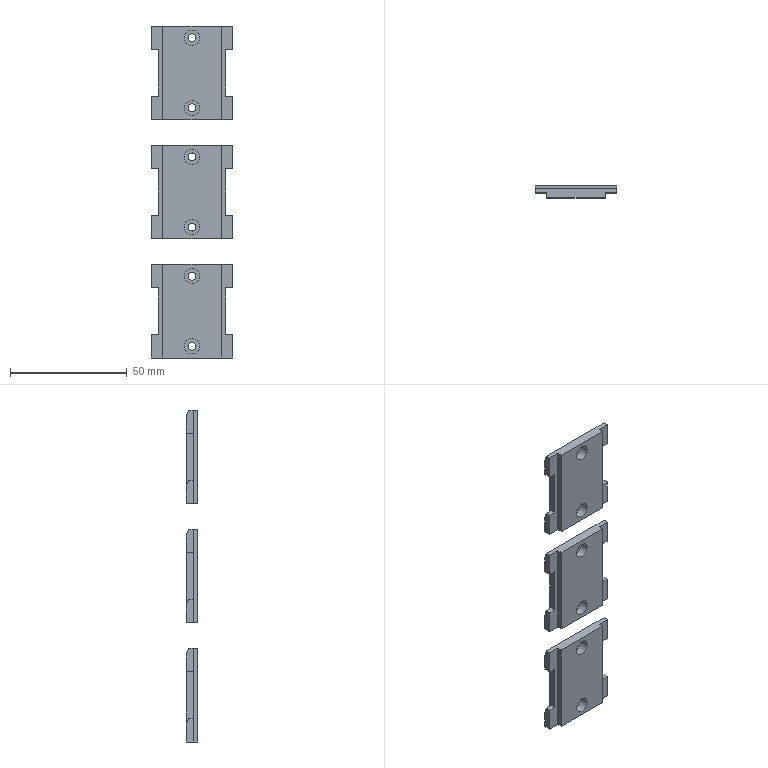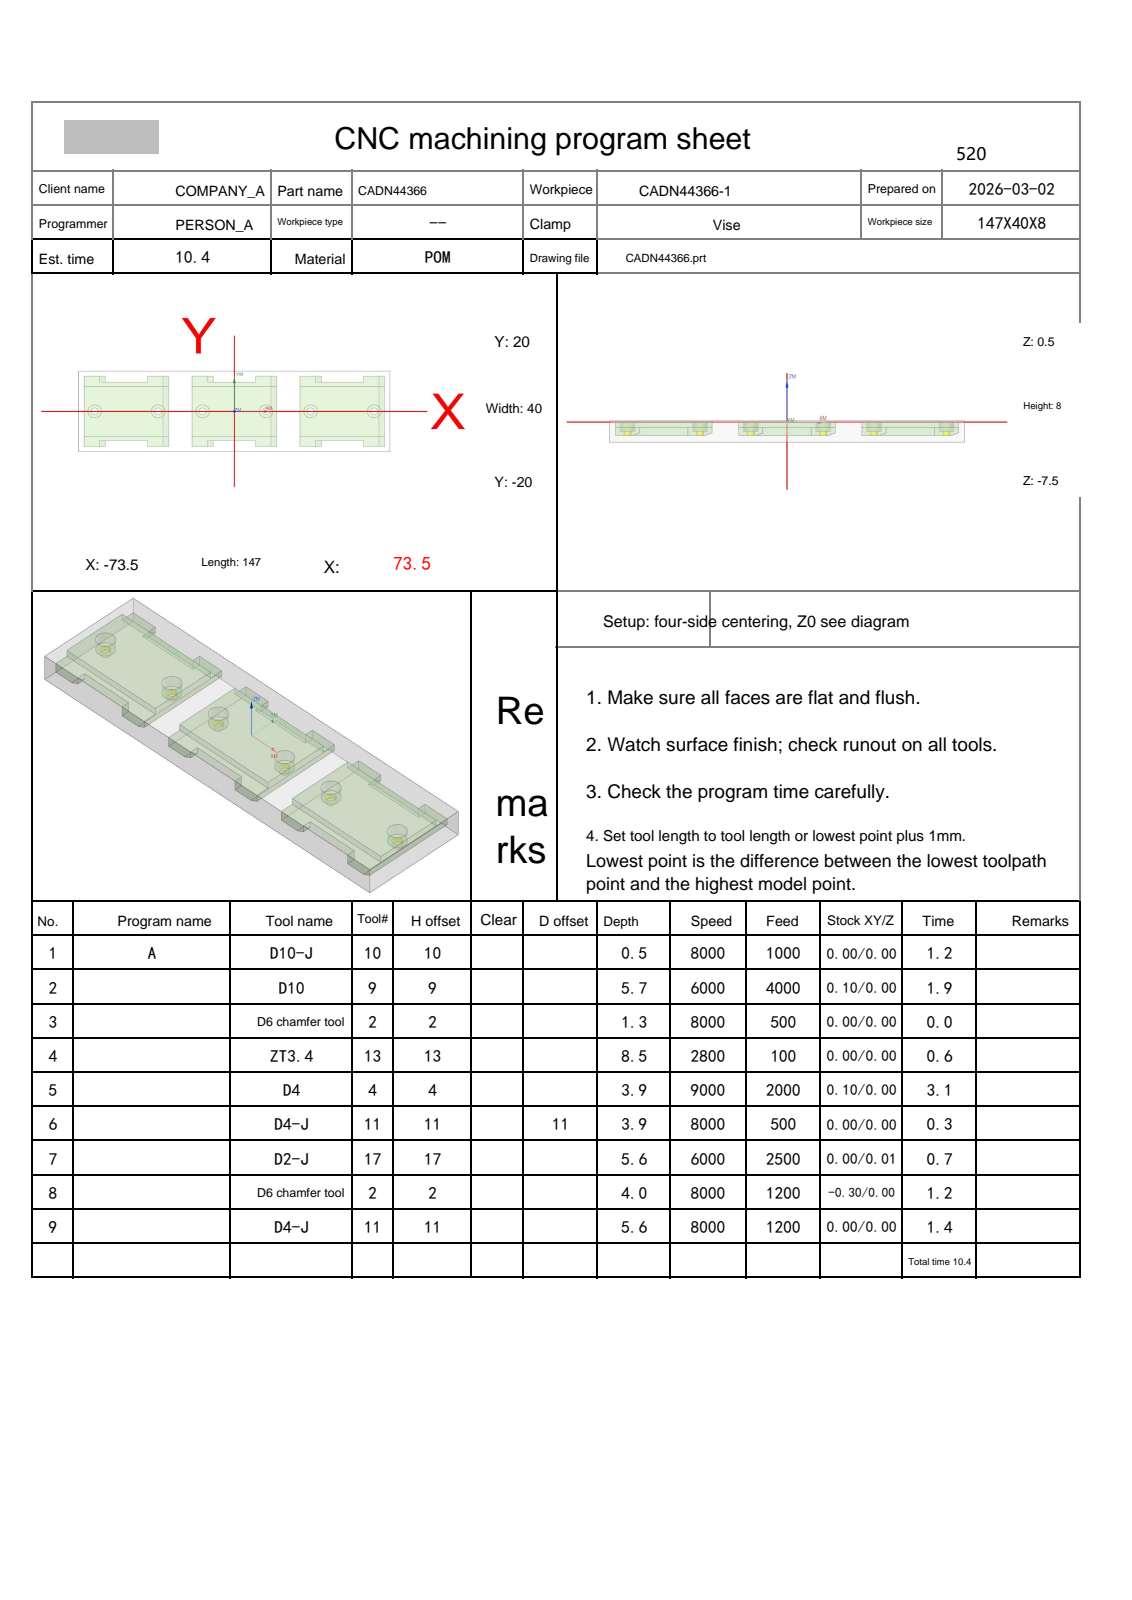NC program | NX | posted by the shop | part box 35 x 5 x 142 mm
Lines 1789 to 2800 of 5584:
N7 T17 M06
(D2-J  D=2. R=0. H=17 ce=0.00 di=0.01)
G00 G90 G54 X-60.211 Y19.24 M03 S6000
G43 H17 Z30.
M08
Z-1.35
G01 X-60.217 Y19.231 Z-1.464 F2000.
X-60.232 Y19.208 Z-1.567
X-60.255 Y19.171 Z-1.658
X-60.283 Y19.122 Z-1.74
X-60.314 Y19.062 Z-1.811
X-60.345 Y18.992 Z-1.873
X-60.374 Y18.914 Z-1.926
X-60.399 Y18.83 Z-1.972
X-60.417 Y18.74 Z-2.009
X-60.427 Y18.646 Z-2.039
X-60.425 Y18.551 Z-2.062
X-60.41 Y18.454 Z-2.08
X-60.379 Y18.358 Z-2.091
X-60.33 Y18.263 Z-2.098
X-60.26 Y18.172 Z-2.1
G02 X-60. Y17.5 I-.74 J-.672 F2500.
G01 Y15.5
X-56.318
X-56.304 Y15.512 Z-2.101
X-56.316 Y15.546 Z-2.104
X-56.351 Y15.599 Z-2.108
X-56.408 Y15.67 Z-2.113
X-56.539 Y15.813 Z-2.125
X-56.853 Y16.119 Z-2.151
X-57.241 Y16.463 Z-2.181
X-57.684 Y16.812 Z-2.215
X-58.154 Y17.145 Z-2.25
X-58.635 Y17.45 Z-2.285
X-59.113 Y17.717 Z-2.319
X-59.51 Y17.909 Z-2.346
X-59.731 Y18.007 Z-2.361
X-60.067 Y18.139 Z-2.384
X-60.161 Y18.169 Z-2.391
X-60.227 Y18.185 Z-2.396
X-60.261 Y18.187 Z-2.399
X-60.26 Y18.172 Z-2.4
G02 X-60. Y17.5 I-.74 J-.672
G01 Y15.5
X-56.318
X-56.304 Y15.512 Z-2.401
X-56.316 Y15.546 Z-2.404
X-56.351 Y15.599 Z-2.408
X-56.408 Y15.67 Z-2.413
X-56.539 Y15.813 Z-2.425
X-56.853 Y16.119 Z-2.451
X-57.241 Y16.463 Z-2.481
X-57.684 Y16.812 Z-2.515
X-58.154 Y17.145 Z-2.55
X-58.635 Y17.45 Z-2.585
X-59.113 Y17.717 Z-2.619
X-59.51 Y17.909 Z-2.646
X-59.731 Y18.007 Z-2.661
X-60.067 Y18.139 Z-2.684
X-60.161 Y18.169 Z-2.691
X-60.227 Y18.185 Z-2.696
X-60.261 Y18.187 Z-2.699
X-60.26 Y18.172 Z-2.7
G02 X-60. Y17.5 I-.74 J-.672
G01 Y15.5
X-56.318
X-56.304 Y15.512 Z-2.701
X-56.316 Y15.546 Z-2.704
X-56.351 Y15.599 Z-2.708
X-56.408 Y15.67 Z-2.713
X-56.539 Y15.813 Z-2.725
X-56.853 Y16.119 Z-2.751
X-57.241 Y16.463 Z-2.781
X-57.684 Y16.812 Z-2.815
X-58.154 Y17.145 Z-2.85
X-58.635 Y17.45 Z-2.885
X-59.113 Y17.717 Z-2.919
X-59.51 Y17.909 Z-2.946
X-59.731 Y18.007 Z-2.961
X-60.067 Y18.139 Z-2.984
X-60.161 Y18.169 Z-2.991
X-60.227 Y18.185 Z-2.996
X-60.261 Y18.187 Z-2.999
X-60.26 Y18.172 Z-3.
G02 X-60. Y17.5 I-.74 J-.672
G01 Y15.5
X-56.318
X-56.304 Y15.512 Z-3.001
X-56.316 Y15.546 Z-3.004
X-56.351 Y15.599 Z-3.008
X-56.408 Y15.67 Z-3.013
X-56.539 Y15.813 Z-3.025
X-56.853 Y16.119 Z-3.051
X-57.241 Y16.463 Z-3.081
X-57.684 Y16.812 Z-3.115
X-58.154 Y17.145 Z-3.15
X-58.635 Y17.45 Z-3.185
X-59.113 Y17.717 Z-3.219
X-59.51 Y17.909 Z-3.246
X-59.731 Y18.007 Z-3.261
X-60.067 Y18.139 Z-3.284
X-60.161 Y18.169 Z-3.291
X-60.227 Y18.185 Z-3.296
X-60.261 Y18.187 Z-3.299
X-60.26 Y18.172 Z-3.3
G02 X-60. Y17.5 I-.74 J-.672
G01 Y15.5
X-56.318
X-56.304 Y15.512 Z-3.301
X-56.316 Y15.546 Z-3.304
X-56.351 Y15.599 Z-3.308
X-56.408 Y15.67 Z-3.313
X-56.539 Y15.813 Z-3.325
X-56.853 Y16.119 Z-3.351
X-57.241 Y16.463 Z-3.381
X-57.684 Y16.812 Z-3.415
X-58.154 Y17.145 Z-3.45
X-58.635 Y17.45 Z-3.485
X-59.113 Y17.717 Z-3.519
X-59.51 Y17.909 Z-3.546
X-59.731 Y18.007 Z-3.561
X-60.067 Y18.139 Z-3.584
X-60.161 Y18.169 Z-3.591
X-60.227 Y18.185 Z-3.596
X-60.261 Y18.187 Z-3.599
X-60.26 Y18.172 Z-3.6
G02 X-60. Y17.5 I-.74 J-.672
G01 Y15.5
X-56.318
X-56.304 Y15.512 Z-3.601
X-56.316 Y15.546 Z-3.604
X-56.351 Y15.599 Z-3.608
X-56.408 Y15.67 Z-3.613
X-56.539 Y15.813 Z-3.625
X-56.853 Y16.119 Z-3.651
X-57.241 Y16.463 Z-3.681
X-57.684 Y16.812 Z-3.715
X-58.154 Y17.145 Z-3.75
X-58.635 Y17.45 Z-3.785
X-59.113 Y17.717 Z-3.819
X-59.51 Y17.909 Z-3.846
X-59.731 Y18.007 Z-3.861
X-60.067 Y18.139 Z-3.884
X-60.161 Y18.169 Z-3.891
X-60.227 Y18.185 Z-3.896
X-60.261 Y18.187 Z-3.899
X-60.26 Y18.172 Z-3.9
G02 X-60. Y17.5 I-.74 J-.672
G01 Y15.5
X-56.318
X-56.304 Y15.512 Z-3.901
X-56.316 Y15.546 Z-3.904
X-56.351 Y15.599 Z-3.908
X-56.408 Y15.67 Z-3.913
X-56.539 Y15.813 Z-3.925
X-56.853 Y16.119 Z-3.951
X-57.241 Y16.463 Z-3.981
X-57.684 Y16.812 Z-4.015
X-58.154 Y17.145 Z-4.05
X-58.635 Y17.45 Z-4.085
X-59.113 Y17.717 Z-4.119
X-59.51 Y17.909 Z-4.146
X-59.731 Y18.007 Z-4.161
X-60.067 Y18.139 Z-4.184
X-60.161 Y18.169 Z-4.191
X-60.227 Y18.185 Z-4.196
X-60.261 Y18.187 Z-4.199
X-60.26 Y18.172 Z-4.2
G02 X-60. Y17.5 I-.74 J-.672
G01 Y15.5
X-56.318
X-56.304 Y15.512 Z-4.201
X-56.316 Y15.546 Z-4.204
X-56.351 Y15.599 Z-4.208
X-56.408 Y15.67 Z-4.213
X-56.539 Y15.813 Z-4.225
X-56.853 Y16.119 Z-4.251
X-57.241 Y16.463 Z-4.281
X-57.684 Y16.812 Z-4.315
X-58.154 Y17.145 Z-4.35
X-58.635 Y17.45 Z-4.385
X-59.113 Y17.717 Z-4.419
X-59.51 Y17.909 Z-4.446
X-59.731 Y18.007 Z-4.461
X-60.067 Y18.139 Z-4.484
X-60.161 Y18.169 Z-4.491
X-60.227 Y18.185 Z-4.496
X-60.261 Y18.187 Z-4.499
X-60.26 Y18.172 Z-4.5
G02 X-60. Y17.5 I-.74 J-.672
G01 Y15.5
X-56.318
X-56.304 Y15.512 Z-4.501
X-56.316 Y15.546 Z-4.504
X-56.351 Y15.599 Z-4.508
X-56.408 Y15.67 Z-4.513
X-56.539 Y15.813 Z-4.525
X-56.853 Y16.119 Z-4.551
X-57.241 Y16.463 Z-4.581
X-57.684 Y16.812 Z-4.615
X-58.154 Y17.145 Z-4.65
X-58.635 Y17.45 Z-4.685
X-59.113 Y17.717 Z-4.719
X-59.51 Y17.909 Z-4.746
X-59.731 Y18.007 Z-4.761
X-60.067 Y18.139 Z-4.784
X-60.161 Y18.169 Z-4.791
X-60.227 Y18.185 Z-4.796
X-60.261 Y18.187 Z-4.799
X-60.26 Y18.172 Z-4.8
G02 X-60. Y17.5 I-.74 J-.672
G01 Y15.5
X-56.318
X-56.304 Y15.512 Z-4.801
X-56.316 Y15.546 Z-4.804
X-56.351 Y15.599 Z-4.808
X-56.408 Y15.67 Z-4.813
X-56.539 Y15.813 Z-4.825
X-56.853 Y16.119 Z-4.851
X-57.241 Y16.463 Z-4.881
X-57.684 Y16.812 Z-4.915
X-58.154 Y17.145 Z-4.95
X-58.635 Y17.45 Z-4.985
X-59.113 Y17.717 Z-5.019
X-59.51 Y17.909 Z-5.046
X-59.731 Y18.007 Z-5.061
X-60.067 Y18.139 Z-5.084
X-60.161 Y18.169 Z-5.091
X-60.227 Y18.185 Z-5.096
X-60.261 Y18.187 Z-5.099
X-60.26 Y18.172 Z-5.1
G02 X-60. Y17.5 I-.74 J-.672
G01 Y15.5
X-56.318
X-56.204 Y15.51 Z-5.098
X-56.101 Y15.536 Z-5.091
X-56.01 Y15.578 Z-5.08
X-55.928 Y15.632 Z-5.062
X-55.857 Y15.694 Z-5.039
X-55.795 Y15.764 Z-5.009
X-55.741 Y15.838 Z-4.972
X-55.696 Y15.912 Z-4.926
X-55.659 Y15.986 Z-4.873
X-55.629 Y16.056 Z-4.811
X-55.606 Y16.118 Z-4.74
X-55.588 Y16.172 Z-4.658
X-55.577 Y16.214 Z-4.567
X-55.57 Y16.24 Z-4.464
X-55.568 Y16.25 Z-4.35
G00 Z3.
X-46.432
Z-1.35
G01 X-46.43 Y16.24 Z-1.464 F2000.
X-46.423 Y16.214 Z-1.567
X-46.412 Y16.172 Z-1.658
X-46.394 Y16.118 Z-1.74
X-46.371 Y16.056 Z-1.811
X-46.341 Y15.986 Z-1.873
X-46.304 Y15.912 Z-1.926
X-46.259 Y15.838 Z-1.972
X-46.205 Y15.764 Z-2.009
X-46.143 Y15.694 Z-2.039
X-46.072 Y15.632 Z-2.062
X-45.99 Y15.578 Z-2.08
X-45.899 Y15.536 Z-2.091
X-45.796 Y15.51 Z-2.098
X-45.682 Y15.5 Z-2.1
X-42. F2500.
Y17.5
G02 X-41.74 Y18.172 I1. J0.0
G01 X-41.739 Y18.187 Z-2.101
X-41.774 Y18.185 Z-2.104
X-41.84 Y18.169 Z-2.109
X-41.936 Y18.14 Z-2.116
X-42.203 Y18.039 Z-2.134
X-42.496 Y17.912 Z-2.154
X-42.895 Y17.721 Z-2.181
X-43.277 Y17.51 Z-2.208
X-43.663 Y17.274 Z-2.236
X-44.044 Y17.018 Z-2.264
X-44.413 Y16.746 Z-2.292
X-44.809 Y16.426 Z-2.322
X-45.16 Y16.111 Z-2.35
X-45.463 Y15.814 Z-2.375
X-45.593 Y15.671 Z-2.387
X-45.649 Y15.599 Z-2.392
X-45.684 Y15.546 Z-2.396
X-45.696 Y15.512 Z-2.399
X-45.682 Y15.5 Z-2.4
X-42.
Y17.5
G02 X-41.74 Y18.172 I1. J0.0
G01 X-41.739 Y18.187 Z-2.401
X-41.774 Y18.185 Z-2.404
X-41.84 Y18.169 Z-2.409
X-41.936 Y18.14 Z-2.416
X-42.203 Y18.039 Z-2.434
X-42.496 Y17.912 Z-2.454
X-42.895 Y17.721 Z-2.481
X-43.277 Y17.51 Z-2.508
X-43.663 Y17.274 Z-2.536
X-44.044 Y17.018 Z-2.564
X-44.413 Y16.746 Z-2.592
X-44.809 Y16.426 Z-2.622
X-45.16 Y16.111 Z-2.65
X-45.463 Y15.814 Z-2.675
X-45.593 Y15.671 Z-2.687
X-45.649 Y15.599 Z-2.692
X-45.684 Y15.546 Z-2.696
X-45.696 Y15.512 Z-2.699
X-45.682 Y15.5 Z-2.7
X-42.
Y17.5
G02 X-41.74 Y18.172 I1. J0.0
G01 X-41.739 Y18.187 Z-2.701
X-41.774 Y18.185 Z-2.704
X-41.84 Y18.169 Z-2.709
X-41.936 Y18.14 Z-2.716
X-42.203 Y18.039 Z-2.734
X-42.496 Y17.912 Z-2.754
X-42.895 Y17.721 Z-2.781
X-43.277 Y17.51 Z-2.808
X-43.663 Y17.274 Z-2.836
X-44.044 Y17.018 Z-2.864
X-44.413 Y16.746 Z-2.892
X-44.809 Y16.426 Z-2.922
X-45.16 Y16.111 Z-2.95
X-45.463 Y15.814 Z-2.975
X-45.593 Y15.671 Z-2.987
X-45.649 Y15.599 Z-2.992
X-45.684 Y15.546 Z-2.996
X-45.696 Y15.512 Z-2.999
X-45.682 Y15.5 Z-3.
X-42.
Y17.5
G02 X-41.74 Y18.172 I1. J0.0
G01 X-41.739 Y18.187 Z-3.001
X-41.774 Y18.185 Z-3.004
X-41.84 Y18.169 Z-3.009
X-41.936 Y18.14 Z-3.016
X-42.203 Y18.039 Z-3.034
X-42.496 Y17.912 Z-3.054
X-42.895 Y17.721 Z-3.081
X-43.277 Y17.51 Z-3.108
X-43.663 Y17.274 Z-3.136
X-44.044 Y17.018 Z-3.164
X-44.413 Y16.746 Z-3.192
X-44.809 Y16.426 Z-3.222
X-45.16 Y16.111 Z-3.25
X-45.463 Y15.814 Z-3.275
X-45.593 Y15.671 Z-3.287
X-45.649 Y15.599 Z-3.292
X-45.684 Y15.546 Z-3.296
X-45.696 Y15.512 Z-3.299
X-45.682 Y15.5 Z-3.3
X-42.
Y17.5
G02 X-41.74 Y18.172 I1. J0.0
G01 X-41.739 Y18.187 Z-3.301
X-41.774 Y18.185 Z-3.304
X-41.84 Y18.169 Z-3.309
X-41.936 Y18.14 Z-3.316
X-42.203 Y18.039 Z-3.334
X-42.496 Y17.912 Z-3.354
X-42.895 Y17.721 Z-3.381
X-43.277 Y17.51 Z-3.408
X-43.663 Y17.274 Z-3.436
X-44.044 Y17.018 Z-3.464
X-44.413 Y16.746 Z-3.492
X-44.809 Y16.426 Z-3.522
X-45.16 Y16.111 Z-3.55
X-45.463 Y15.814 Z-3.575
X-45.593 Y15.671 Z-3.587
X-45.649 Y15.599 Z-3.592
X-45.684 Y15.546 Z-3.596
X-45.696 Y15.512 Z-3.599
X-45.682 Y15.5 Z-3.6
X-42.
Y17.5
G02 X-41.74 Y18.172 I1. J0.0
G01 X-41.739 Y18.187 Z-3.601
X-41.774 Y18.185 Z-3.604
X-41.84 Y18.169 Z-3.609
X-41.936 Y18.14 Z-3.616
X-42.203 Y18.039 Z-3.634
X-42.496 Y17.912 Z-3.654
X-42.895 Y17.721 Z-3.681
X-43.277 Y17.51 Z-3.708
X-43.663 Y17.274 Z-3.736
X-44.044 Y17.018 Z-3.764
X-44.413 Y16.746 Z-3.792
X-44.809 Y16.426 Z-3.822
X-45.16 Y16.111 Z-3.85
X-45.463 Y15.814 Z-3.875
X-45.593 Y15.671 Z-3.887
X-45.649 Y15.599 Z-3.892
X-45.684 Y15.546 Z-3.896
X-45.696 Y15.512 Z-3.899
X-45.682 Y15.5 Z-3.9
X-42.
Y17.5
G02 X-41.74 Y18.172 I1. J0.0
G01 X-41.739 Y18.187 Z-3.901
X-41.774 Y18.185 Z-3.904
X-41.84 Y18.169 Z-3.909
X-41.936 Y18.14 Z-3.916
X-42.203 Y18.039 Z-3.934
X-42.496 Y17.912 Z-3.954
X-42.895 Y17.721 Z-3.981
X-43.277 Y17.51 Z-4.008
X-43.663 Y17.274 Z-4.036
X-44.044 Y17.018 Z-4.064
X-44.413 Y16.746 Z-4.092
X-44.809 Y16.426 Z-4.122
X-45.16 Y16.111 Z-4.15
X-45.463 Y15.814 Z-4.175
X-45.593 Y15.671 Z-4.187
X-45.649 Y15.599 Z-4.192
X-45.684 Y15.546 Z-4.196
X-45.696 Y15.512 Z-4.199
X-45.682 Y15.5 Z-4.2
X-42.
Y17.5
G02 X-41.74 Y18.172 I1. J0.0
G01 X-41.739 Y18.187 Z-4.201
X-41.774 Y18.185 Z-4.204
X-41.84 Y18.169 Z-4.209
X-41.936 Y18.14 Z-4.216
X-42.203 Y18.039 Z-4.234
X-42.496 Y17.912 Z-4.254
X-42.895 Y17.721 Z-4.281
X-43.277 Y17.51 Z-4.308
X-43.663 Y17.274 Z-4.336
X-44.044 Y17.018 Z-4.364
X-44.413 Y16.746 Z-4.392
X-44.809 Y16.426 Z-4.422
X-45.16 Y16.111 Z-4.45
X-45.463 Y15.814 Z-4.475
X-45.593 Y15.671 Z-4.487
X-45.649 Y15.599 Z-4.492
X-45.684 Y15.546 Z-4.496
X-45.696 Y15.512 Z-4.499
X-45.682 Y15.5 Z-4.5
X-42.
Y17.5
G02 X-41.74 Y18.172 I1. J0.0
G01 X-41.739 Y18.187 Z-4.501
X-41.774 Y18.185 Z-4.504
X-41.84 Y18.169 Z-4.509
X-41.936 Y18.14 Z-4.516
X-42.203 Y18.039 Z-4.534
X-42.496 Y17.912 Z-4.554
X-42.895 Y17.721 Z-4.581
X-43.277 Y17.51 Z-4.608
X-43.663 Y17.274 Z-4.636
X-44.044 Y17.018 Z-4.664
X-44.413 Y16.746 Z-4.692
X-44.809 Y16.426 Z-4.722
X-45.16 Y16.111 Z-4.75
X-45.463 Y15.814 Z-4.775
X-45.593 Y15.671 Z-4.787
X-45.649 Y15.599 Z-4.792
X-45.684 Y15.546 Z-4.796
X-45.696 Y15.512 Z-4.799
X-45.682 Y15.5 Z-4.8
X-42.
Y17.5
G02 X-41.74 Y18.172 I1. J0.0
G01 X-41.739 Y18.187 Z-4.801
X-41.774 Y18.185 Z-4.804
X-41.84 Y18.169 Z-4.809
X-41.936 Y18.14 Z-4.816
X-42.203 Y18.039 Z-4.834
X-42.496 Y17.912 Z-4.854
X-42.895 Y17.721 Z-4.881
X-43.278 Y17.51 Z-4.908
X-43.663 Y17.274 Z-4.936
X-44.044 Y17.018 Z-4.964
X-44.413 Y16.746 Z-4.992
X-44.809 Y16.426 Z-5.022
X-45.16 Y16.111 Z-5.05
X-45.463 Y15.814 Z-5.075
X-45.593 Y15.671 Z-5.087
X-45.649 Y15.599 Z-5.092
X-45.684 Y15.546 Z-5.096
X-45.696 Y15.512 Z-5.099
X-45.682 Y15.5 Z-5.1
X-42.
Y17.5
G02 X-41.74 Y18.172 I1. J0.0
G01 X-41.671 Y18.264 Z-5.098
X-41.623 Y18.359 Z-5.091
X-41.595 Y18.456 Z-5.08
X-41.582 Y18.554 Z-5.062
X-41.584 Y18.652 Z-5.039
X-41.598 Y18.747 Z-5.009
X-41.62 Y18.838 Z-4.972
X-41.65 Y18.925 Z-4.926
X-41.683 Y19.004 Z-4.873
X-41.718 Y19.076 Z-4.811
X-41.752 Y19.138 Z-4.74
X-41.783 Y19.189 Z-4.658
X-41.808 Y19.227 Z-4.567
X-41.825 Y19.251 Z-4.464
X-41.831 Y19.259 Z-4.35
G00 Z30.
X-41.789 Y-19.24
Z-1.35
G01 X-41.783 Y-19.231 Z-1.464 F2000.
X-41.768 Y-19.208 Z-1.567
X-41.745 Y-19.171 Z-1.658
X-41.717 Y-19.122 Z-1.74
X-41.686 Y-19.062 Z-1.811
X-41.655 Y-18.992 Z-1.873
X-41.626 Y-18.914 Z-1.926
X-41.601 Y-18.83 Z-1.972
X-41.583 Y-18.74 Z-2.009
X-41.573 Y-18.646 Z-2.039
X-41.575 Y-18.551 Z-2.062
X-41.59 Y-18.454 Z-2.08
X-41.621 Y-18.358 Z-2.091
X-41.67 Y-18.263 Z-2.098
X-41.74 Y-18.172 Z-2.1
G02 X-42. Y-17.5 I.74 J.672 F2500.
G01 Y-15.5
X-45.682
X-45.696 Y-15.512 Z-2.101
X-45.684 Y-15.546 Z-2.104
X-45.649 Y-15.599 Z-2.108
X-45.592 Y-15.67 Z-2.113
X-45.461 Y-15.813 Z-2.125
X-45.147 Y-16.119 Z-2.151
X-44.759 Y-16.463 Z-2.181
X-44.316 Y-16.812 Z-2.215
X-43.846 Y-17.145 Z-2.25
X-43.365 Y-17.45 Z-2.285
X-42.887 Y-17.717 Z-2.319
X-42.49 Y-17.909 Z-2.346
X-42.269 Y-18.007 Z-2.361
X-41.933 Y-18.139 Z-2.384
X-41.839 Y-18.169 Z-2.391
X-41.773 Y-18.185 Z-2.396
X-41.739 Y-18.187 Z-2.399
X-41.74 Y-18.172 Z-2.4
G02 X-42. Y-17.5 I.74 J.672
G01 Y-15.5
X-45.682
X-45.696 Y-15.512 Z-2.401
X-45.684 Y-15.546 Z-2.404
X-45.649 Y-15.599 Z-2.408
X-45.592 Y-15.67 Z-2.413
X-45.461 Y-15.813 Z-2.425
X-45.147 Y-16.119 Z-2.451
X-44.759 Y-16.463 Z-2.481
X-44.316 Y-16.812 Z-2.515
X-43.846 Y-17.145 Z-2.55
X-43.365 Y-17.45 Z-2.585
X-42.887 Y-17.717 Z-2.619
X-42.49 Y-17.909 Z-2.646
X-42.269 Y-18.007 Z-2.661
X-41.933 Y-18.139 Z-2.684
X-41.839 Y-18.169 Z-2.691
X-41.773 Y-18.185 Z-2.696
X-41.739 Y-18.187 Z-2.699
X-41.74 Y-18.172 Z-2.7
G02 X-42. Y-17.5 I.74 J.672
G01 Y-15.5
X-45.682
X-45.696 Y-15.512 Z-2.701
X-45.684 Y-15.546 Z-2.704
X-45.649 Y-15.599 Z-2.708
X-45.592 Y-15.67 Z-2.713
X-45.461 Y-15.813 Z-2.725
X-45.147 Y-16.119 Z-2.751
X-44.759 Y-16.463 Z-2.781
X-44.316 Y-16.812 Z-2.815
X-43.846 Y-17.145 Z-2.85
X-43.365 Y-17.45 Z-2.885
X-42.887 Y-17.717 Z-2.919
X-42.49 Y-17.909 Z-2.946
X-42.269 Y-18.007 Z-2.961
X-41.933 Y-18.139 Z-2.984
X-41.839 Y-18.169 Z-2.991
X-41.773 Y-18.185 Z-2.996
X-41.739 Y-18.187 Z-2.999
X-41.74 Y-18.172 Z-3.
G02 X-42. Y-17.5 I.74 J.672
G01 Y-15.5
X-45.682
X-45.696 Y-15.512 Z-3.001
X-45.684 Y-15.546 Z-3.004
X-45.649 Y-15.599 Z-3.008
X-45.592 Y-15.67 Z-3.013
X-45.461 Y-15.813 Z-3.025
X-45.147 Y-16.119 Z-3.051
X-44.759 Y-16.463 Z-3.081
X-44.316 Y-16.812 Z-3.115
X-43.846 Y-17.145 Z-3.15
X-43.365 Y-17.45 Z-3.185
X-42.887 Y-17.717 Z-3.219
X-42.49 Y-17.909 Z-3.246
X-42.269 Y-18.007 Z-3.261
X-41.933 Y-18.139 Z-3.284
X-41.839 Y-18.169 Z-3.291
X-41.773 Y-18.185 Z-3.296
X-41.739 Y-18.187 Z-3.299
X-41.74 Y-18.172 Z-3.3
G02 X-42. Y-17.5 I.74 J.672
G01 Y-15.5
X-45.682
X-45.696 Y-15.512 Z-3.301
X-45.684 Y-15.546 Z-3.304
X-45.649 Y-15.599 Z-3.308
X-45.592 Y-15.67 Z-3.313
X-45.461 Y-15.813 Z-3.325
X-45.147 Y-16.119 Z-3.351
X-44.759 Y-16.463 Z-3.381
X-44.316 Y-16.812 Z-3.415
X-43.846 Y-17.145 Z-3.45
X-43.365 Y-17.45 Z-3.485
X-42.887 Y-17.717 Z-3.519
X-42.49 Y-17.909 Z-3.546
X-42.269 Y-18.007 Z-3.561
X-41.933 Y-18.139 Z-3.584
X-41.839 Y-18.169 Z-3.591
X-41.773 Y-18.185 Z-3.596
X-41.739 Y-18.187 Z-3.599
X-41.74 Y-18.172 Z-3.6
G02 X-42. Y-17.5 I.74 J.672
G01 Y-15.5
X-45.682
X-45.696 Y-15.512 Z-3.601
X-45.684 Y-15.546 Z-3.604
X-45.649 Y-15.599 Z-3.608
X-45.592 Y-15.67 Z-3.613
X-45.461 Y-15.813 Z-3.625
X-45.147 Y-16.119 Z-3.651
X-44.759 Y-16.463 Z-3.681
X-44.316 Y-16.812 Z-3.715
X-43.846 Y-17.145 Z-3.75
X-43.365 Y-17.45 Z-3.785
X-42.887 Y-17.717 Z-3.819
X-42.49 Y-17.909 Z-3.846
X-42.269 Y-18.007 Z-3.861
X-41.933 Y-18.139 Z-3.884
X-41.839 Y-18.169 Z-3.891
X-41.773 Y-18.185 Z-3.896
X-41.739 Y-18.187 Z-3.899
X-41.74 Y-18.172 Z-3.9
G02 X-42. Y-17.5 I.74 J.672
G01 Y-15.5
X-45.682
X-45.696 Y-15.512 Z-3.901
X-45.684 Y-15.546 Z-3.904
X-45.649 Y-15.599 Z-3.908
X-45.592 Y-15.67 Z-3.913
X-45.461 Y-15.813 Z-3.925
X-45.147 Y-16.119 Z-3.951
X-44.759 Y-16.463 Z-3.981
X-44.316 Y-16.812 Z-4.015
X-43.846 Y-17.145 Z-4.05
X-43.365 Y-17.45 Z-4.085
X-42.887 Y-17.717 Z-4.119
X-42.49 Y-17.909 Z-4.146
X-42.269 Y-18.007 Z-4.161
X-41.933 Y-18.139 Z-4.184
X-41.839 Y-18.169 Z-4.191
X-41.773 Y-18.185 Z-4.196
X-41.739 Y-18.187 Z-4.199
X-41.74 Y-18.172 Z-4.2
G02 X-42. Y-17.5 I.74 J.672
G01 Y-15.5
X-45.682
X-45.696 Y-15.512 Z-4.201
X-45.684 Y-15.546 Z-4.204
X-45.649 Y-15.599 Z-4.208
X-45.592 Y-15.67 Z-4.213
X-45.461 Y-15.813 Z-4.225
X-45.147 Y-16.119 Z-4.251
X-44.759 Y-16.463 Z-4.281
X-44.316 Y-16.812 Z-4.315
X-43.846 Y-17.145 Z-4.35
X-43.365 Y-17.45 Z-4.385
X-42.887 Y-17.717 Z-4.419
X-42.49 Y-17.909 Z-4.446
X-42.269 Y-18.007 Z-4.461
X-41.933 Y-18.139 Z-4.484
X-41.839 Y-18.169 Z-4.491
X-41.773 Y-18.185 Z-4.496
X-41.739 Y-18.187 Z-4.499
X-41.74 Y-18.172 Z-4.5
G02 X-42. Y-17.5 I.74 J.672
G01 Y-15.5
X-45.682
X-45.696 Y-15.512 Z-4.501
X-45.684 Y-15.546 Z-4.504
X-45.649 Y-15.599 Z-4.508
X-45.592 Y-15.67 Z-4.513
X-45.461 Y-15.813 Z-4.525
X-45.147 Y-16.119 Z-4.551
X-44.759 Y-16.463 Z-4.581
X-44.316 Y-16.812 Z-4.615
X-43.846 Y-17.145 Z-4.65
X-43.365 Y-17.45 Z-4.685
X-42.887 Y-17.717 Z-4.719
X-42.49 Y-17.909 Z-4.746
X-42.269 Y-18.007 Z-4.761
X-41.933 Y-18.139 Z-4.784
X-41.839 Y-18.169 Z-4.791
X-41.773 Y-18.185 Z-4.796
X-41.739 Y-18.187 Z-4.799
X-41.74 Y-18.172 Z-4.8
G02 X-42. Y-17.5 I.74 J.672
G01 Y-15.5
X-45.682
X-45.696 Y-15.512 Z-4.801
X-45.684 Y-15.546 Z-4.804
X-45.649 Y-15.599 Z-4.808
X-45.592 Y-15.67 Z-4.813
X-45.461 Y-15.813 Z-4.825
X-45.147 Y-16.119 Z-4.851
X-44.759 Y-16.463 Z-4.881
X-44.316 Y-16.812 Z-4.915
X-43.846 Y-17.145 Z-4.95
X-43.365 Y-17.45 Z-4.985
X-42.887 Y-17.717 Z-5.019
X-42.49 Y-17.909 Z-5.046
X-42.268 Y-18.007 Z-5.061
X-41.933 Y-18.139 Z-5.084
X-41.839 Y-18.169 Z-5.091
X-41.773 Y-18.185 Z-5.096
X-41.739 Y-18.187 Z-5.099
X-41.74 Y-18.172 Z-5.1
G02 X-42. Y-17.5 I.74 J.672
G01 Y-15.5
X-45.682
X-45.796 Y-15.51 Z-5.098
X-45.899 Y-15.536 Z-5.091
X-45.991 Y-15.578 Z-5.08
X-46.072 Y-15.632 Z-5.062
X-46.143 Y-15.694 Z-5.039
X-46.205 Y-15.764 Z-5.009
X-46.259 Y-15.838 Z-4.972
X-46.304 Y-15.912 Z-4.926
X-46.341 Y-15.986 Z-4.873
X-46.371 Y-16.056 Z-4.811
X-46.394 Y-16.118 Z-4.74
X-46.412 Y-16.172 Z-4.658
X-46.423 Y-16.214 Z-4.567
X-46.43 Y-16.24 Z-4.464
X-46.432 Y-16.25 Z-4.35
G00 Z3.
X-55.568
Z-1.35
G01 X-55.57 Y-16.24 Z-1.464 F2000.
X-55.577 Y-16.214 Z-1.567
X-55.588 Y-16.172 Z-1.658
X-55.606 Y-16.118 Z-1.74
X-55.629 Y-16.056 Z-1.811
X-55.659 Y-15.986 Z-1.873
X-55.696 Y-15.912 Z-1.926
X-55.741 Y-15.838 Z-1.972
X-55.795 Y-15.764 Z-2.009
X-55.857 Y-15.694 Z-2.039
X-55.928 Y-15.632 Z-2.062
X-56.01 Y-15.578 Z-2.08
X-56.101 Y-15.536 Z-2.091
X-56.204 Y-15.51 Z-2.098
X-56.318 Y-15.5 Z-2.1
X-60. F2500.
Y-17.5
G02 X-60.26 Y-18.172 I-1. J0.0
G01 X-60.261 Y-18.187 Z-2.101
X-60.226 Y-18.185 Z-2.104
X-60.159 Y-18.169 Z-2.109
X-60.064 Y-18.14 Z-2.116
X-59.797 Y-18.039 Z-2.134
X-59.503 Y-17.912 Z-2.154
X-59.105 Y-17.721 Z-2.181
X-58.722 Y-17.511 Z-2.208
X-58.337 Y-17.274 Z-2.236
X-57.956 Y-17.018 Z-2.264
X-57.587 Y-16.746 Z-2.292
X-57.191 Y-16.427 Z-2.322
X-56.84 Y-16.111 Z-2.35
X-56.537 Y-15.814 Z-2.375
X-56.407 Y-15.671 Z-2.387
X-56.351 Y-15.599 Z-2.392
X-56.316 Y-15.546 Z-2.396
X-56.304 Y-15.512 Z-2.399
X-56.318 Y-15.5 Z-2.4
X-60.
Y-17.5
G02 X-60.26 Y-18.172 I-1. J0.0
G01 X-60.261 Y-18.187 Z-2.401
X-60.226 Y-18.185 Z-2.404
X-60.159 Y-18.169 Z-2.409
X-60.064 Y-18.14 Z-2.416
X-59.797 Y-18.039 Z-2.434
X-59.503 Y-17.912 Z-2.454
X-59.105 Y-17.721 Z-2.481
X-58.722 Y-17.511 Z-2.508
X-58.337 Y-17.274 Z-2.536
X-57.956 Y-17.018 Z-2.564
X-57.587 Y-16.746 Z-2.592
X-57.191 Y-16.427 Z-2.622
X-56.84 Y-16.111 Z-2.65
X-56.537 Y-15.814 Z-2.675
X-56.407 Y-15.671 Z-2.687
X-56.351 Y-15.599 Z-2.692
X-56.316 Y-15.546 Z-2.696
X-56.304 Y-15.512 Z-2.699
X-56.318 Y-15.5 Z-2.7
X-60.
Y-17.5
G02 X-60.26 Y-18.172 I-1. J0.0
G01 X-60.261 Y-18.187 Z-2.701
X-60.226 Y-18.185 Z-2.704
X-60.159 Y-18.169 Z-2.709
X-60.064 Y-18.14 Z-2.716
X-59.797 Y-18.039 Z-2.734
X-59.503 Y-17.912 Z-2.754
X-59.105 Y-17.721 Z-2.781
X-58.722 Y-17.511 Z-2.808
X-58.337 Y-17.274 Z-2.836
X-57.956 Y-17.018 Z-2.864
X-57.587 Y-16.746 Z-2.892
X-57.191 Y-16.427 Z-2.922
X-56.84 Y-16.111 Z-2.95
X-56.537 Y-15.814 Z-2.975
X-56.407 Y-15.671 Z-2.987
X-56.351 Y-15.599 Z-2.992
X-56.316 Y-15.546 Z-2.996
X-56.304 Y-15.512 Z-2.999
X-56.318 Y-15.5 Z-3.
X-60.
Y-17.5
G02 X-60.26 Y-18.172 I-1. J0.0
G01 X-60.261 Y-18.187 Z-3.001
X-60.226 Y-18.185 Z-3.004
X-60.159 Y-18.169 Z-3.009
X-60.064 Y-18.14 Z-3.016
X-59.797 Y-18.039 Z-3.034
X-59.503 Y-17.912 Z-3.054
X-59.105 Y-17.721 Z-3.081
X-58.722 Y-17.511 Z-3.108
X-58.337 Y-17.274 Z-3.136
X-57.956 Y-17.018 Z-3.164
X-57.587 Y-16.746 Z-3.192
X-57.191 Y-16.427 Z-3.222
X-56.84 Y-16.111 Z-3.25
X-56.537 Y-15.814 Z-3.275
X-56.407 Y-15.671 Z-3.287
X-56.351 Y-15.599 Z-3.292
X-56.316 Y-15.546 Z-3.296
X-56.304 Y-15.512 Z-3.299
X-56.318 Y-15.5 Z-3.3
X-60.
Y-17.5
G02 X-60.26 Y-18.172 I-1. J0.0
G01 X-60.261 Y-18.187 Z-3.301
X-60.226 Y-18.185 Z-3.304
X-60.159 Y-18.169 Z-3.309
X-60.064 Y-18.14 Z-3.316
X-59.797 Y-18.039 Z-3.334
X-59.503 Y-17.912 Z-3.354
X-59.105 Y-17.721 Z-3.381
X-58.722 Y-17.511 Z-3.408
X-58.337 Y-17.274 Z-3.436
X-57.956 Y-17.018 Z-3.464
X-57.587 Y-16.746 Z-3.492
X-57.191 Y-16.427 Z-3.522
X-56.84 Y-16.111 Z-3.55
X-56.537 Y-15.814 Z-3.575
X-56.407 Y-15.671 Z-3.587
X-56.351 Y-15.599 Z-3.592
X-56.316 Y-15.546 Z-3.596
X-56.304 Y-15.512 Z-3.599
X-56.318 Y-15.5 Z-3.6
X-60.
Y-17.5
G02 X-60.26 Y-18.172 I-1. J0.0
G01 X-60.261 Y-18.187 Z-3.601
X-60.226 Y-18.185 Z-3.604
X-60.159 Y-18.169 Z-3.609
X-60.064 Y-18.14 Z-3.616
X-59.797 Y-18.039 Z-3.634
X-59.503 Y-17.912 Z-3.654
X-59.105 Y-17.721 Z-3.681
X-58.722 Y-17.511 Z-3.708
X-58.337 Y-17.274 Z-3.736
X-57.956 Y-17.018 Z-3.764
X-57.587 Y-16.746 Z-3.792
X-57.191 Y-16.427 Z-3.822
X-56.84 Y-16.111 Z-3.85
X-56.537 Y-15.814 Z-3.875
X-56.407 Y-15.671 Z-3.887
X-56.351 Y-15.599 Z-3.892
X-56.316 Y-15.546 Z-3.896
X-56.304 Y-15.512 Z-3.899
X-56.318 Y-15.5 Z-3.9
X-60.
Y-17.5
G02 X-60.26 Y-18.172 I-1. J0.0
G01 X-60.261 Y-18.187 Z-3.901
X-60.226 Y-18.185 Z-3.904
X-60.159 Y-18.169 Z-3.909
X-60.064 Y-18.14 Z-3.916
X-59.797 Y-18.039 Z-3.934
X-59.503 Y-17.912 Z-3.954
X-59.105 Y-17.721 Z-3.981
X-58.722 Y-17.511 Z-4.008
X-58.337 Y-17.274 Z-4.036
X-57.956 Y-17.018 Z-4.064
X-57.587 Y-16.746 Z-4.092
X-57.191 Y-16.427 Z-4.122
X-56.84 Y-16.111 Z-4.15
X-56.537 Y-15.814 Z-4.175
X-56.407 Y-15.671 Z-4.187
X-56.351 Y-15.599 Z-4.192
X-56.316 Y-15.546 Z-4.196
X-56.304 Y-15.512 Z-4.199
X-56.318 Y-15.5 Z-4.2
X-60.
Y-17.5
G02 X-60.26 Y-18.172 I-1. J0.0
G01 X-60.261 Y-18.187 Z-4.201
X-60.226 Y-18.185 Z-4.204
X-60.159 Y-18.169 Z-4.209
X-60.064 Y-18.14 Z-4.216
X-59.797 Y-18.039 Z-4.234
X-59.503 Y-17.912 Z-4.254
X-59.105 Y-17.721 Z-4.281
X-58.722 Y-17.511 Z-4.308
X-58.337 Y-17.274 Z-4.336
X-57.956 Y-17.018 Z-4.364
X-57.587 Y-16.746 Z-4.392
X-57.191 Y-16.427 Z-4.422
X-56.84 Y-16.111 Z-4.45
X-56.537 Y-15.814 Z-4.475
X-56.407 Y-15.671 Z-4.487
X-56.351 Y-15.599 Z-4.492
X-56.316 Y-15.546 Z-4.496
X-56.304 Y-15.512 Z-4.499
X-56.318 Y-15.5 Z-4.5
X-60.
Y-17.5
G02 X-60.26 Y-18.172 I-1. J0.0
G01 X-60.261 Y-18.187 Z-4.501
X-60.226 Y-18.185 Z-4.504
X-60.159 Y-18.169 Z-4.509
X-60.064 Y-18.14 Z-4.516
X-59.797 Y-18.039 Z-4.534
X-59.503 Y-17.912 Z-4.554
X-59.105 Y-17.721 Z-4.581
X-58.722 Y-17.511 Z-4.608
X-58.337 Y-17.274 Z-4.636
X-57.956 Y-17.018 Z-4.664
X-57.587 Y-16.746 Z-4.692
X-57.191 Y-16.427 Z-4.722
X-56.84 Y-16.111 Z-4.75
X-56.537 Y-15.814 Z-4.775
X-56.407 Y-15.671 Z-4.787
X-56.351 Y-15.599 Z-4.792
X-56.316 Y-15.546 Z-4.796
X-56.304 Y-15.512 Z-4.799
X-56.318 Y-15.5 Z-4.8
X-60.
Y-17.5
G02 X-60.26 Y-18.172 I-1. J0.0
G01 X-60.261 Y-18.187 Z-4.801
X-60.226 Y-18.185 Z-4.804
X-60.159 Y-18.169 Z-4.809
X-60.064 Y-18.14 Z-4.816
X-59.797 Y-18.039 Z-4.834
X-59.503 Y-17.912 Z-4.854
X-59.105 Y-17.721 Z-4.881
X-58.722 Y-17.511 Z-4.908
X-58.337 Y-17.274 Z-4.936
X-57.956 Y-17.018 Z-4.964
X-57.587 Y-16.746 Z-4.992
X-57.191 Y-16.427 Z-5.022
X-56.84 Y-16.111 Z-5.05
X-56.537 Y-15.814 Z-5.075
X-56.407 Y-15.671 Z-5.087
X-56.351 Y-15.599 Z-5.092
X-56.316 Y-15.546 Z-5.096
X-56.304 Y-15.512 Z-5.099
X-56.318 Y-15.5 Z-5.1
X-60.
Y-17.5
G02 X-60.26 Y-18.172 I-1. J0.0
G01 X-60.329 Y-18.264 Z-5.098
X-60.377 Y-18.359 Z-5.091
X-60.405 Y-18.456 Z-5.08
X-60.417 Y-18.554 Z-5.062
X-60.415 Y-18.652 Z-5.039
X-60.402 Y-18.747 Z-5.009
X-60.379 Y-18.839 Z-4.972
X-60.35 Y-18.925 Z-4.926
X-60.316 Y-19.005 Z-4.873
X-60.281 Y-19.076 Z-4.811
X-60.247 Y-19.138 Z-4.74
X-60.216 Y-19.189 Z-4.658
X-60.191 Y-19.227 Z-4.567
X-60.174 Y-19.251 Z-4.464
X-60.168 Y-19.259 Z-4.35
G00 Z30.
X-9.211 Y19.24
Z-1.35
G01 X-9.217 Y19.231 Z-1.464 F2000.
X-9.232 Y19.208 Z-1.567